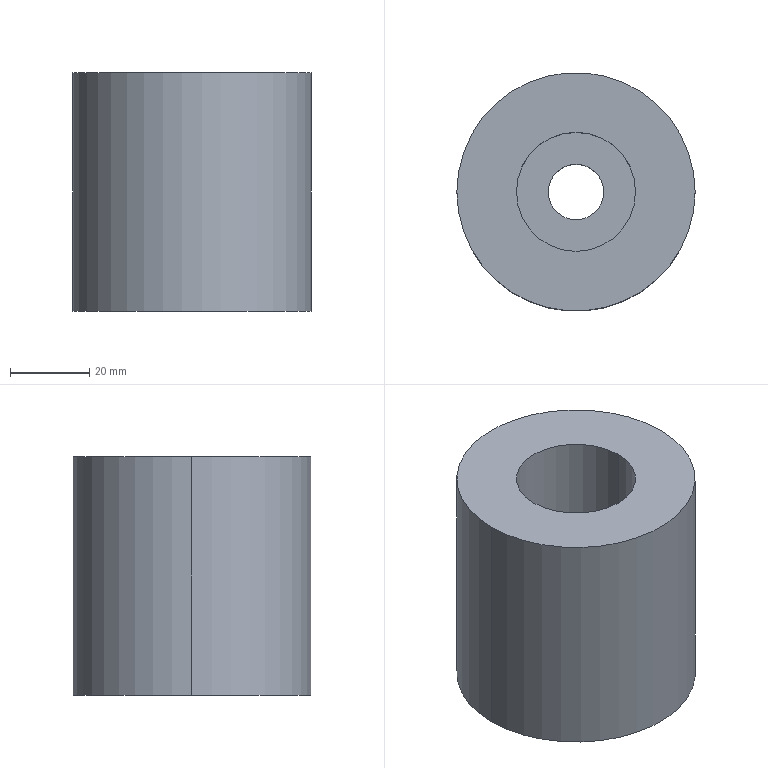Part | SolidWorks | features ICE 2, Extrusion 1 | 1 solid | 9 faces | box 60 x 60 x 60 mm | volume 143822 mm3 | cylinder 6 | plane 3 | commonest cylinder face diameters 14 x2 30 x2 60 x2
STEP:
#1=CARTESIAN_POINT('',(-15.,0.,30.));
#2=VERTEX_POINT('',#1);
#3=CARTESIAN_POINT('',(15.,0.,30.));
#4=VERTEX_POINT('',#3);
#5=CARTESIAN_POINT('',(0.,0.,30.));
#6=DIRECTION('',(0.,0.,1.));
#7=DIRECTION('',(1.,0.,0.));
#8=AXIS2_PLACEMENT_3D('',#5,#6,#7);
#9=CIRCLE('',#8,15.);
#10=EDGE_CURVE('',#2,#4,#9,.T.);
#11=ORIENTED_EDGE('',*,*,#10,.F.);
#12=CARTESIAN_POINT('',(-15.,0.,60.));
#13=VERTEX_POINT('',#12);
#14=CARTESIAN_POINT('',(-15.,0.,30.));
#15=DIRECTION('',(0.,0.,1.));
#16=VECTOR('',#15,1000.);
#17=LINE('',#14,#16);
#18=EDGE_CURVE('',#2,#13,#17,.T.);
#19=ORIENTED_EDGE('',*,*,#18,.T.);
#20=CARTESIAN_POINT('',(15.,0.,60.));
#21=VERTEX_POINT('',#20);
#22=CARTESIAN_POINT('',(0.,0.,60.));
#23=DIRECTION('',(0.,0.,1.));
#24=DIRECTION('',(1.,0.,0.));
#25=AXIS2_PLACEMENT_3D('',#22,#23,#24);
#26=CIRCLE('',#25,15.);
#27=EDGE_CURVE('',#13,#21,#26,.T.);
#28=ORIENTED_EDGE('',*,*,#27,.T.);
#29=CARTESIAN_POINT('',(15.,0.,30.));
#30=DIRECTION('',(0.,0.,1.));
#31=VECTOR('',#30,1000.);
#32=LINE('',#29,#31);
#33=EDGE_CURVE('',#4,#21,#32,.T.);
#34=ORIENTED_EDGE('',*,*,#33,.F.);
#35=EDGE_LOOP('',(#11,#19,#28,#34));
#36=FACE_OUTER_BOUND('',#35,.T.);
#37=CARTESIAN_POINT('',(0.,0.,30.));
#38=DIRECTION('',(0.,0.,1.));
#39=DIRECTION('',(1.,0.,0.));
#40=AXIS2_PLACEMENT_3D('',#37,#38,#39);
#41=CYLINDRICAL_SURFACE('',#40,15.);
#42=ADVANCED_FACE('',(#36),#41,.F.);
#43=CARTESIAN_POINT('',(30.,0.,60.));
#44=VERTEX_POINT('',#43);
#45=CARTESIAN_POINT('',(-30.,0.,60.));
#46=VERTEX_POINT('',#45);
#47=CARTESIAN_POINT('',(0.,0.,60.));
#48=DIRECTION('',(0.,0.,1.));
#49=DIRECTION('',(1.,0.,0.));
#50=AXIS2_PLACEMENT_3D('',#47,#48,#49);
#51=CIRCLE('',#50,30.);
#52=EDGE_CURVE('',#44,#46,#51,.T.);
#53=ORIENTED_EDGE('',*,*,#52,.F.);
#54=CARTESIAN_POINT('',(30.,0.,0.));
#55=VERTEX_POINT('',#54);
#56=CARTESIAN_POINT('',(30.,0.,60.));
#57=DIRECTION('',(0.,0.,-1.));
#58=VECTOR('',#57,1000.);
#59=LINE('',#56,#58);
#60=EDGE_CURVE('',#44,#55,#59,.T.);
#61=ORIENTED_EDGE('',*,*,#60,.T.);
#62=CARTESIAN_POINT('',(-30.,0.,0.));
#63=VERTEX_POINT('',#62);
#64=CARTESIAN_POINT('',(0.,0.,0.));
#65=DIRECTION('',(0.,0.,1.));
#66=DIRECTION('',(1.,0.,0.));
#67=AXIS2_PLACEMENT_3D('',#64,#65,#66);
#68=CIRCLE('',#67,30.);
#69=EDGE_CURVE('',#55,#63,#68,.T.);
#70=ORIENTED_EDGE('',*,*,#69,.T.);
#71=CARTESIAN_POINT('',(-30.,0.,60.));
#72=DIRECTION('',(0.,0.,-1.));
#73=VECTOR('',#72,1000.);
#74=LINE('',#71,#73);
#75=EDGE_CURVE('',#46,#63,#74,.T.);
#76=ORIENTED_EDGE('',*,*,#75,.F.);
#77=EDGE_LOOP('',(#53,#61,#70,#76));
#78=FACE_OUTER_BOUND('',#77,.T.);
#79=CARTESIAN_POINT('',(0.,0.,60.));
#80=DIRECTION('',(0.,0.,-1.));
#81=DIRECTION('',(-1.,0.,0.));
#82=AXIS2_PLACEMENT_3D('',#79,#80,#81);
#83=CYLINDRICAL_SURFACE('',#82,30.);
#84=ADVANCED_FACE('',(#78),#83,.T.);
#85=CARTESIAN_POINT('',(-7.,0.,0.));
#86=VERTEX_POINT('',#85);
#87=CARTESIAN_POINT('',(7.,0.,0.));
#88=VERTEX_POINT('',#87);
#89=CARTESIAN_POINT('',(0.,0.,0.));
#90=DIRECTION('',(0.,0.,1.));
#91=DIRECTION('',(1.,0.,0.));
#92=AXIS2_PLACEMENT_3D('',#89,#90,#91);
#93=CIRCLE('',#92,7.);
#94=EDGE_CURVE('',#86,#88,#93,.T.);
#95=ORIENTED_EDGE('',*,*,#94,.F.);
#96=CARTESIAN_POINT('',(-7.,0.,30.));
#97=VERTEX_POINT('',#96);
#98=CARTESIAN_POINT('',(-7.,0.,0.));
#99=DIRECTION('',(0.,0.,1.));
#100=VECTOR('',#99,1000.);
#101=LINE('',#98,#100);
#102=EDGE_CURVE('',#86,#97,#101,.T.);
#103=ORIENTED_EDGE('',*,*,#102,.T.);
#104=CARTESIAN_POINT('',(7.,0.,30.));
#105=VERTEX_POINT('',#104);
#106=CARTESIAN_POINT('',(0.,0.,30.));
#107=DIRECTION('',(0.,0.,-1.));
#108=DIRECTION('',(1.,0.,0.));
#109=AXIS2_PLACEMENT_3D('',#106,#107,#108);
#110=CIRCLE('',#109,7.);
#111=EDGE_CURVE('',#105,#97,#110,.T.);
#112=ORIENTED_EDGE('',*,*,#111,.F.);
#113=CARTESIAN_POINT('',(7.,0.,0.));
#114=DIRECTION('',(0.,0.,1.));
#115=VECTOR('',#114,1000.);
#116=LINE('',#113,#115);
#117=EDGE_CURVE('',#88,#105,#116,.T.);
#118=ORIENTED_EDGE('',*,*,#117,.F.);
#119=EDGE_LOOP('',(#95,#103,#112,#118));
#120=FACE_OUTER_BOUND('',#119,.T.);
#121=CARTESIAN_POINT('',(0.,0.,0.));
#122=DIRECTION('',(0.,0.,1.));
#123=DIRECTION('',(1.,0.,0.));
#124=AXIS2_PLACEMENT_3D('',#121,#122,#123);
#125=CYLINDRICAL_SURFACE('',#124,7.);
#126=ADVANCED_FACE('',(#120),#125,.F.);
#127=ORIENTED_EDGE('',*,*,#102,.F.);
#128=CARTESIAN_POINT('',(0.,0.,0.));
#129=DIRECTION('',(0.,0.,1.));
#130=DIRECTION('',(1.,0.,0.));
#131=AXIS2_PLACEMENT_3D('',#128,#129,#130);
#132=CIRCLE('',#131,7.);
#133=EDGE_CURVE('',#88,#86,#132,.T.);
#134=ORIENTED_EDGE('',*,*,#133,.F.);
#135=ORIENTED_EDGE('',*,*,#117,.T.);
#136=CARTESIAN_POINT('',(0.,0.,30.));
#137=DIRECTION('',(0.,0.,-1.));
#138=DIRECTION('',(1.,0.,0.));
#139=AXIS2_PLACEMENT_3D('',#136,#137,#138);
#140=CIRCLE('',#139,7.);
#141=EDGE_CURVE('',#97,#105,#140,.T.);
#142=ORIENTED_EDGE('',*,*,#141,.F.);
#143=EDGE_LOOP('',(#127,#134,#135,#142));
#144=FACE_OUTER_BOUND('',#143,.T.);
#145=CARTESIAN_POINT('',(0.,0.,0.));
#146=DIRECTION('',(0.,0.,1.));
#147=DIRECTION('',(1.,0.,0.));
#148=AXIS2_PLACEMENT_3D('',#145,#146,#147);
#149=CYLINDRICAL_SURFACE('',#148,7.);
#150=ADVANCED_FACE('',(#144),#149,.F.);
#151=ORIENTED_EDGE('',*,*,#60,.F.);
#152=CARTESIAN_POINT('',(0.,0.,60.));
#153=DIRECTION('',(0.,0.,1.));
#154=DIRECTION('',(1.,0.,0.));
#155=AXIS2_PLACEMENT_3D('',#152,#153,#154);
#156=CIRCLE('',#155,30.);
#157=EDGE_CURVE('',#46,#44,#156,.T.);
#158=ORIENTED_EDGE('',*,*,#157,.F.);
#159=ORIENTED_EDGE('',*,*,#75,.T.);
#160=CARTESIAN_POINT('',(0.,0.,0.));
#161=DIRECTION('',(0.,0.,1.));
#162=DIRECTION('',(1.,0.,0.));
#163=AXIS2_PLACEMENT_3D('',#160,#161,#162);
#164=CIRCLE('',#163,30.);
#165=EDGE_CURVE('',#63,#55,#164,.T.);
#166=ORIENTED_EDGE('',*,*,#165,.T.);
#167=EDGE_LOOP('',(#151,#158,#159,#166));
#168=FACE_OUTER_BOUND('',#167,.T.);
#169=CARTESIAN_POINT('',(0.,0.,60.));
#170=DIRECTION('',(0.,0.,-1.));
#171=DIRECTION('',(-1.,0.,0.));
#172=AXIS2_PLACEMENT_3D('',#169,#170,#171);
#173=CYLINDRICAL_SURFACE('',#172,30.);
#174=ADVANCED_FACE('',(#168),#173,.T.);
#175=CARTESIAN_POINT('',(0.,0.,60.));
#176=DIRECTION('',(0.,0.,1.));
#177=DIRECTION('',(1.,0.,0.));
#178=AXIS2_PLACEMENT_3D('',#175,#176,#177);
#179=CIRCLE('',#178,15.);
#180=EDGE_CURVE('',#21,#13,#179,.T.);
#181=ORIENTED_EDGE('',*,*,#180,.F.);
#182=ORIENTED_EDGE('',*,*,#27,.F.);
#183=EDGE_LOOP('',(#181,#182));
#184=FACE_BOUND('',#183,.T.);
#185=ORIENTED_EDGE('',*,*,#157,.T.);
#186=ORIENTED_EDGE('',*,*,#52,.T.);
#187=EDGE_LOOP('',(#185,#186));
#188=FACE_OUTER_BOUND('',#187,.T.);
#189=CARTESIAN_POINT('',(0.,0.,60.));
#190=DIRECTION('',(0.,0.,1.));
#191=DIRECTION('',(1.,0.,0.));
#192=AXIS2_PLACEMENT_3D('',#189,#190,#191);
#193=PLANE('',#192);
#194=ADVANCED_FACE('',(#184,#188),#193,.T.);
#195=ORIENTED_EDGE('',*,*,#133,.T.);
#196=ORIENTED_EDGE('',*,*,#94,.T.);
#197=EDGE_LOOP('',(#195,#196));
#198=FACE_BOUND('',#197,.T.);
#199=ORIENTED_EDGE('',*,*,#165,.F.);
#200=ORIENTED_EDGE('',*,*,#69,.F.);
#201=EDGE_LOOP('',(#199,#200));
#202=FACE_OUTER_BOUND('',#201,.T.);
#203=CARTESIAN_POINT('',(0.,0.,0.));
#204=DIRECTION('',(0.,0.,1.));
#205=DIRECTION('',(1.,0.,0.));
#206=AXIS2_PLACEMENT_3D('',#203,#204,#205);
#207=PLANE('',#206);
#208=ADVANCED_FACE('',(#198,#202),#207,.F.);
#209=CARTESIAN_POINT('',(0.,0.,30.));
#210=DIRECTION('',(0.,0.,1.));
#211=DIRECTION('',(1.,0.,0.));
#212=AXIS2_PLACEMENT_3D('',#209,#210,#211);
#213=CIRCLE('',#212,15.);
#214=EDGE_CURVE('',#4,#2,#213,.T.);
#215=ORIENTED_EDGE('',*,*,#214,.T.);
#216=ORIENTED_EDGE('',*,*,#10,.T.);
#217=EDGE_LOOP('',(#215,#216));
#218=FACE_OUTER_BOUND('',#217,.T.);
#219=ORIENTED_EDGE('',*,*,#111,.T.);
#220=ORIENTED_EDGE('',*,*,#141,.T.);
#221=EDGE_LOOP('',(#219,#220));
#222=FACE_BOUND('',#221,.T.);
#223=CARTESIAN_POINT('',(0.,0.,30.));
#224=DIRECTION('',(0.,0.,1.));
#225=DIRECTION('',(1.,0.,0.));
#226=AXIS2_PLACEMENT_3D('',#223,#224,#225);
#227=PLANE('',#226);
#228=ADVANCED_FACE('',(#218,#222),#227,.T.);
#229=ORIENTED_EDGE('',*,*,#18,.F.);
#230=ORIENTED_EDGE('',*,*,#214,.F.);
#231=ORIENTED_EDGE('',*,*,#33,.T.);
#232=ORIENTED_EDGE('',*,*,#180,.T.);
#233=EDGE_LOOP('',(#229,#230,#231,#232));
#234=FACE_OUTER_BOUND('',#233,.T.);
#235=CARTESIAN_POINT('',(0.,0.,30.));
#236=DIRECTION('',(0.,0.,1.));
#237=DIRECTION('',(1.,0.,0.));
#238=AXIS2_PLACEMENT_3D('',#235,#236,#237);
#239=CYLINDRICAL_SURFACE('',#238,15.);
#240=ADVANCED_FACE('',(#234),#239,.F.);
#241=CLOSED_SHELL('',(#42,#84,#126,#150,#174,#194,#208,#228,#240));
#242=MANIFOLD_SOLID_BREP('',#241);
#243=CARTESIAN_POINT('',(0.,0.,0.));
#244=DIRECTION('',(0.,0.,1.));
#245=DIRECTION('',(1.,0.,0.));
#246=AXIS2_PLACEMENT_3D('',#243,#244,#245);
#247=(LENGTH_UNIT()NAMED_UNIT(*)SI_UNIT(.MILLI.,.METRE.));
#248=UNCERTAINTY_MEASURE_WITH_UNIT(LENGTH_MEASURE(0.00001),#247,'','');
#249=(NAMED_UNIT(*)PLANE_ANGLE_UNIT()SI_UNIT($,.RADIAN.));
#250=(NAMED_UNIT(*)SI_UNIT($,.STERADIAN.)SOLID_ANGLE_UNIT());
#251=(GEOMETRIC_REPRESENTATION_CONTEXT(3)GLOBAL_UNCERTAINTY_ASSIGNED_CONTEXT((#248))GLOBAL_UNIT_ASSIGNED_CONTEXT((#247,#249,#250))REPRESENTATION_CONTEXT('',''));
#252=ADVANCED_BREP_SHAPE_REPRESENTATION('',(#242,#246),#251);